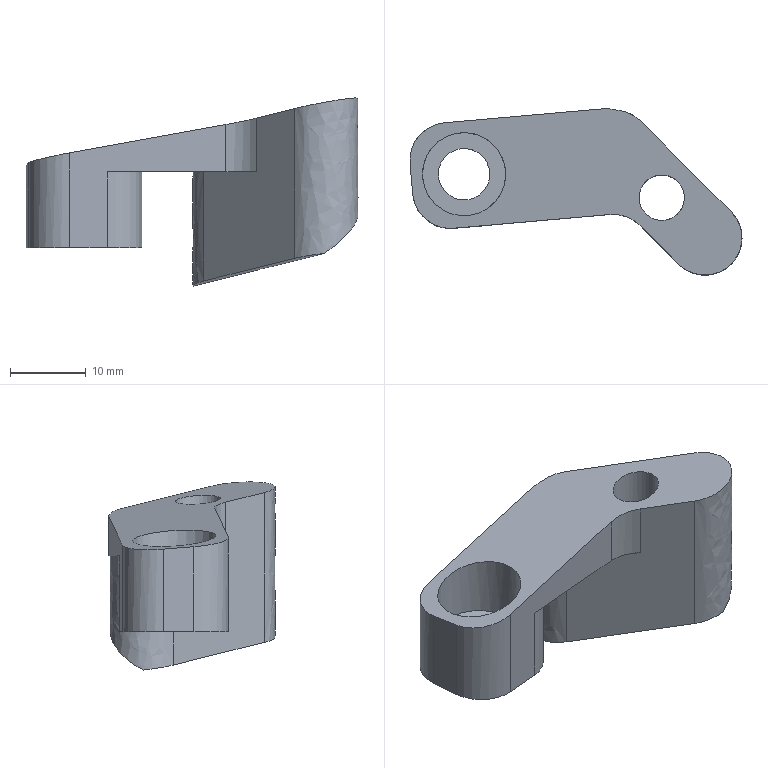Part | STEP file | gslz 2016.10.28-13_id1650_x_t | 1 solid | 23 faces | box 43.888 x 21.981 x 24.856 mm | volume 5888 mm3 | plane 12 | cylinder 9 | spline 2 | commonest cylinder face diameters 10 x6 6 x1 6.8 x1 11 x1